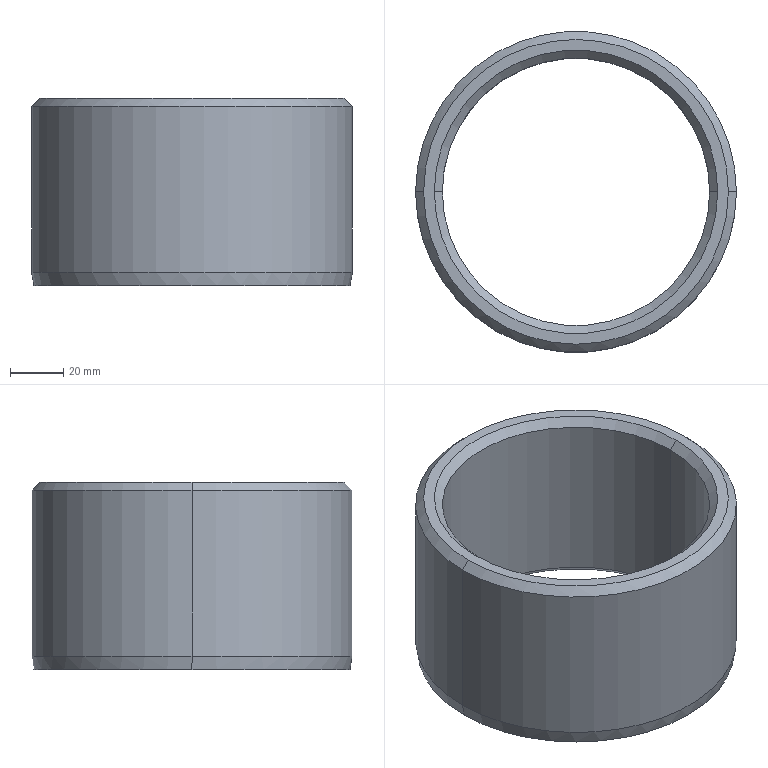Part | SolidWorks | features Chamfer 2, Extrusion 1 | 1 solid | 14 faces | box 120 x 120 x 70 mm | volume 236524 mm3 | cone 8 | cylinder 4 | plane 2 | commonest cylinder face diameters 100 x2 120 x2
STEP:
#1=CARTESIAN_POINT('',(-59.118,0.,-35.));
#2=VERTEX_POINT('',#1);
#3=CARTESIAN_POINT('',(59.118,0.,-35.));
#4=VERTEX_POINT('',#3);
#5=CARTESIAN_POINT('',(0.,0.,-35.));
#6=DIRECTION('',(0.,0.,-1.));
#7=DIRECTION('',(1.,0.,0.));
#8=AXIS2_PLACEMENT_3D('',#5,#6,#7);
#9=CIRCLE('',#8,59.118);
#10=EDGE_CURVE('',#2,#4,#9,.T.);
#11=ORIENTED_EDGE('',*,*,#10,.F.);
#12=CARTESIAN_POINT('',(-60.,0.,-30.));
#13=VERTEX_POINT('',#12);
#14=CARTESIAN_POINT('',(-60.,0.,-30.));
#15=DIRECTION('',(-0.1736,0.,0.9848));
#16=VECTOR('',#15,1000.);
#17=LINE('',#14,#16);
#18=EDGE_CURVE('',#2,#13,#17,.T.);
#19=ORIENTED_EDGE('',*,*,#18,.T.);
#20=CARTESIAN_POINT('',(60.,0.,-30.));
#21=VERTEX_POINT('',#20);
#22=CARTESIAN_POINT('',(0.,0.,-30.));
#23=DIRECTION('',(0.,0.,1.));
#24=DIRECTION('',(1.,0.,0.));
#25=AXIS2_PLACEMENT_3D('',#22,#23,#24);
#26=CIRCLE('',#25,60.);
#27=EDGE_CURVE('',#21,#13,#26,.T.);
#28=ORIENTED_EDGE('',*,*,#27,.F.);
#29=CARTESIAN_POINT('',(60.,0.,-30.));
#30=DIRECTION('',(0.1736,0.,0.9848));
#31=VECTOR('',#30,1000.);
#32=LINE('',#29,#31);
#33=EDGE_CURVE('',#4,#21,#32,.T.);
#34=ORIENTED_EDGE('',*,*,#33,.F.);
#35=EDGE_LOOP('',(#11,#19,#28,#34));
#36=FACE_OUTER_BOUND('',#35,.T.);
#37=CARTESIAN_POINT('',(0.,0.,-30.));
#38=DIRECTION('',(0.,0.,1.));
#39=DIRECTION('',(1.,0.,0.));
#40=AXIS2_PLACEMENT_3D('',#37,#38,#39);
#41=CONICAL_SURFACE('',#40,60.,0.1745);
#42=ADVANCED_FACE('',(#36),#41,.T.);
#43=CARTESIAN_POINT('',(57.,0.,35.));
#44=VERTEX_POINT('',#43);
#45=CARTESIAN_POINT('',(-57.,0.,35.));
#46=VERTEX_POINT('',#45);
#47=CARTESIAN_POINT('',(0.,0.,35.));
#48=DIRECTION('',(0.,0.,1.));
#49=DIRECTION('',(1.,0.,0.));
#50=AXIS2_PLACEMENT_3D('',#47,#48,#49);
#51=CIRCLE('',#50,57.);
#52=EDGE_CURVE('',#44,#46,#51,.T.);
#53=ORIENTED_EDGE('',*,*,#52,.F.);
#54=CARTESIAN_POINT('',(60.,0.,32.));
#55=VERTEX_POINT('',#54);
#56=CARTESIAN_POINT('',(57.,0.,35.));
#57=DIRECTION('',(0.7071,0.,-0.7071));
#58=VECTOR('',#57,1000.);
#59=LINE('',#56,#58);
#60=EDGE_CURVE('',#44,#55,#59,.T.);
#61=ORIENTED_EDGE('',*,*,#60,.T.);
#62=CARTESIAN_POINT('',(-60.,0.,32.));
#63=VERTEX_POINT('',#62);
#64=CARTESIAN_POINT('',(0.,0.,32.));
#65=DIRECTION('',(0.,0.,-1.));
#66=DIRECTION('',(1.,0.,0.));
#67=AXIS2_PLACEMENT_3D('',#64,#65,#66);
#68=CIRCLE('',#67,60.);
#69=EDGE_CURVE('',#63,#55,#68,.T.);
#70=ORIENTED_EDGE('',*,*,#69,.F.);
#71=CARTESIAN_POINT('',(-57.,0.,35.));
#72=DIRECTION('',(-0.7071,0.,-0.7071));
#73=VECTOR('',#72,1000.);
#74=LINE('',#71,#73);
#75=EDGE_CURVE('',#46,#63,#74,.T.);
#76=ORIENTED_EDGE('',*,*,#75,.F.);
#77=EDGE_LOOP('',(#53,#61,#70,#76));
#78=FACE_OUTER_BOUND('',#77,.T.);
#79=CARTESIAN_POINT('',(0.,0.,35.));
#80=DIRECTION('',(0.,0.,-1.));
#81=DIRECTION('',(-1.,0.,0.));
#82=AXIS2_PLACEMENT_3D('',#79,#80,#81);
#83=CONICAL_SURFACE('',#82,57.,0.7854);
#84=ADVANCED_FACE('',(#78),#83,.T.);
#85=CARTESIAN_POINT('',(-50.,0.,32.));
#86=VERTEX_POINT('',#85);
#87=CARTESIAN_POINT('',(50.,0.,32.));
#88=VERTEX_POINT('',#87);
#89=CARTESIAN_POINT('',(0.,0.,32.));
#90=DIRECTION('',(0.,0.,1.));
#91=DIRECTION('',(1.,0.,0.));
#92=AXIS2_PLACEMENT_3D('',#89,#90,#91);
#93=CIRCLE('',#92,50.);
#94=EDGE_CURVE('',#86,#88,#93,.T.);
#95=ORIENTED_EDGE('',*,*,#94,.F.);
#96=CARTESIAN_POINT('',(-53.,0.,35.));
#97=VERTEX_POINT('',#96);
#98=CARTESIAN_POINT('',(-50.,0.,32.));
#99=DIRECTION('',(-0.7071,0.,0.7071));
#100=VECTOR('',#99,1000.);
#101=LINE('',#98,#100);
#102=EDGE_CURVE('',#86,#97,#101,.T.);
#103=ORIENTED_EDGE('',*,*,#102,.T.);
#104=CARTESIAN_POINT('',(53.,0.,35.));
#105=VERTEX_POINT('',#104);
#106=CARTESIAN_POINT('',(0.,0.,35.));
#107=DIRECTION('',(0.,0.,-1.));
#108=DIRECTION('',(1.,0.,0.));
#109=AXIS2_PLACEMENT_3D('',#106,#107,#108);
#110=CIRCLE('',#109,53.);
#111=EDGE_CURVE('',#105,#97,#110,.T.);
#112=ORIENTED_EDGE('',*,*,#111,.F.);
#113=CARTESIAN_POINT('',(50.,0.,32.));
#114=DIRECTION('',(0.7071,0.,0.7071));
#115=VECTOR('',#114,1000.);
#116=LINE('',#113,#115);
#117=EDGE_CURVE('',#88,#105,#116,.T.);
#118=ORIENTED_EDGE('',*,*,#117,.F.);
#119=EDGE_LOOP('',(#95,#103,#112,#118));
#120=FACE_OUTER_BOUND('',#119,.T.);
#121=CARTESIAN_POINT('',(0.,0.,32.));
#122=DIRECTION('',(0.,0.,1.));
#123=DIRECTION('',(1.,0.,0.));
#124=AXIS2_PLACEMENT_3D('',#121,#122,#123);
#125=CONICAL_SURFACE('',#124,50.,0.7854);
#126=ADVANCED_FACE('',(#120),#125,.F.);
#127=CARTESIAN_POINT('',(50.,0.,-32.));
#128=VERTEX_POINT('',#127);
#129=CARTESIAN_POINT('',(-50.,0.,-32.));
#130=VERTEX_POINT('',#129);
#131=CARTESIAN_POINT('',(0.,0.,-32.));
#132=DIRECTION('',(0.,0.,-1.));
#133=DIRECTION('',(1.,0.,0.));
#134=AXIS2_PLACEMENT_3D('',#131,#132,#133);
#135=CIRCLE('',#134,50.);
#136=EDGE_CURVE('',#128,#130,#135,.T.);
#137=ORIENTED_EDGE('',*,*,#136,.F.);
#138=CARTESIAN_POINT('',(53.,0.,-35.));
#139=VERTEX_POINT('',#138);
#140=CARTESIAN_POINT('',(53.,0.,-35.));
#141=DIRECTION('',(0.7071,0.,-0.7071));
#142=VECTOR('',#141,1000.);
#143=LINE('',#140,#142);
#144=EDGE_CURVE('',#128,#139,#143,.T.);
#145=ORIENTED_EDGE('',*,*,#144,.T.);
#146=CARTESIAN_POINT('',(-53.,0.,-35.));
#147=VERTEX_POINT('',#146);
#148=CARTESIAN_POINT('',(0.,0.,-35.));
#149=DIRECTION('',(0.,0.,1.));
#150=DIRECTION('',(1.,0.,0.));
#151=AXIS2_PLACEMENT_3D('',#148,#149,#150);
#152=CIRCLE('',#151,53.);
#153=EDGE_CURVE('',#147,#139,#152,.T.);
#154=ORIENTED_EDGE('',*,*,#153,.F.);
#155=CARTESIAN_POINT('',(-53.,0.,-35.));
#156=DIRECTION('',(-0.7071,0.,-0.7071));
#157=VECTOR('',#156,1000.);
#158=LINE('',#155,#157);
#159=EDGE_CURVE('',#130,#147,#158,.T.);
#160=ORIENTED_EDGE('',*,*,#159,.F.);
#161=EDGE_LOOP('',(#137,#145,#154,#160));
#162=FACE_OUTER_BOUND('',#161,.T.);
#163=CARTESIAN_POINT('',(0.,0.,-35.));
#164=DIRECTION('',(0.,0.,-1.));
#165=DIRECTION('',(-1.,0.,0.));
#166=AXIS2_PLACEMENT_3D('',#163,#164,#165);
#167=CONICAL_SURFACE('',#166,53.,0.7854);
#168=ADVANCED_FACE('',(#162),#167,.F.);
#169=ORIENTED_EDGE('',*,*,#94,.T.);
#170=CARTESIAN_POINT('',(50.,0.,35.));
#171=DIRECTION('',(0.,0.,-1.));
#172=VECTOR('',#171,1000.);
#173=LINE('',#170,#172);
#174=EDGE_CURVE('',#88,#128,#173,.T.);
#175=ORIENTED_EDGE('',*,*,#174,.T.);
#176=ORIENTED_EDGE('',*,*,#136,.T.);
#177=CARTESIAN_POINT('',(-50.,0.,35.));
#178=DIRECTION('',(0.,0.,-1.));
#179=VECTOR('',#178,1000.);
#180=LINE('',#177,#179);
#181=EDGE_CURVE('',#86,#130,#180,.T.);
#182=ORIENTED_EDGE('',*,*,#181,.F.);
#183=EDGE_LOOP('',(#169,#175,#176,#182));
#184=FACE_OUTER_BOUND('',#183,.T.);
#185=CARTESIAN_POINT('',(0.,0.,35.));
#186=DIRECTION('',(0.,0.,-1.));
#187=DIRECTION('',(-1.,0.,0.));
#188=AXIS2_PLACEMENT_3D('',#185,#186,#187);
#189=CYLINDRICAL_SURFACE('',#188,50.);
#190=ADVANCED_FACE('',(#184),#189,.F.);
#191=ORIENTED_EDGE('',*,*,#69,.T.);
#192=CARTESIAN_POINT('',(60.,0.,35.));
#193=DIRECTION('',(0.,0.,-1.));
#194=VECTOR('',#193,1000.);
#195=LINE('',#192,#194);
#196=EDGE_CURVE('',#55,#21,#195,.T.);
#197=ORIENTED_EDGE('',*,*,#196,.T.);
#198=ORIENTED_EDGE('',*,*,#27,.T.);
#199=CARTESIAN_POINT('',(-60.,0.,35.));
#200=DIRECTION('',(0.,0.,-1.));
#201=VECTOR('',#200,1000.);
#202=LINE('',#199,#201);
#203=EDGE_CURVE('',#63,#13,#202,.T.);
#204=ORIENTED_EDGE('',*,*,#203,.F.);
#205=EDGE_LOOP('',(#191,#197,#198,#204));
#206=FACE_OUTER_BOUND('',#205,.T.);
#207=CARTESIAN_POINT('',(0.,0.,35.));
#208=DIRECTION('',(0.,0.,-1.));
#209=DIRECTION('',(-1.,0.,0.));
#210=AXIS2_PLACEMENT_3D('',#207,#208,#209);
#211=CYLINDRICAL_SURFACE('',#210,60.);
#212=ADVANCED_FACE('',(#206),#211,.T.);
#213=ORIENTED_EDGE('',*,*,#111,.T.);
#214=CARTESIAN_POINT('',(0.,0.,35.));
#215=DIRECTION('',(0.,0.,-1.));
#216=DIRECTION('',(1.,0.,0.));
#217=AXIS2_PLACEMENT_3D('',#214,#215,#216);
#218=CIRCLE('',#217,53.);
#219=EDGE_CURVE('',#97,#105,#218,.T.);
#220=ORIENTED_EDGE('',*,*,#219,.T.);
#221=EDGE_LOOP('',(#213,#220));
#222=FACE_BOUND('',#221,.T.);
#223=CARTESIAN_POINT('',(0.,0.,35.));
#224=DIRECTION('',(0.,0.,1.));
#225=DIRECTION('',(1.,0.,0.));
#226=AXIS2_PLACEMENT_3D('',#223,#224,#225);
#227=CIRCLE('',#226,57.);
#228=EDGE_CURVE('',#46,#44,#227,.T.);
#229=ORIENTED_EDGE('',*,*,#228,.T.);
#230=ORIENTED_EDGE('',*,*,#52,.T.);
#231=EDGE_LOOP('',(#229,#230));
#232=FACE_OUTER_BOUND('',#231,.T.);
#233=CARTESIAN_POINT('',(0.,0.,35.));
#234=DIRECTION('',(0.,0.,1.));
#235=DIRECTION('',(1.,0.,0.));
#236=AXIS2_PLACEMENT_3D('',#233,#234,#235);
#237=PLANE('',#236);
#238=ADVANCED_FACE('',(#222,#232),#237,.T.);
#239=CARTESIAN_POINT('',(0.,0.,-35.));
#240=DIRECTION('',(0.,0.,-1.));
#241=DIRECTION('',(1.,0.,0.));
#242=AXIS2_PLACEMENT_3D('',#239,#240,#241);
#243=CIRCLE('',#242,59.118);
#244=EDGE_CURVE('',#4,#2,#243,.T.);
#245=ORIENTED_EDGE('',*,*,#244,.T.);
#246=ORIENTED_EDGE('',*,*,#10,.T.);
#247=EDGE_LOOP('',(#245,#246));
#248=FACE_OUTER_BOUND('',#247,.T.);
#249=ORIENTED_EDGE('',*,*,#153,.T.);
#250=CARTESIAN_POINT('',(0.,0.,-35.));
#251=DIRECTION('',(0.,0.,1.));
#252=DIRECTION('',(1.,0.,0.));
#253=AXIS2_PLACEMENT_3D('',#250,#251,#252);
#254=CIRCLE('',#253,53.);
#255=EDGE_CURVE('',#139,#147,#254,.T.);
#256=ORIENTED_EDGE('',*,*,#255,.T.);
#257=EDGE_LOOP('',(#249,#256));
#258=FACE_BOUND('',#257,.T.);
#259=CARTESIAN_POINT('',(0.,0.,-35.));
#260=DIRECTION('',(0.,0.,1.));
#261=DIRECTION('',(1.,0.,0.));
#262=AXIS2_PLACEMENT_3D('',#259,#260,#261);
#263=PLANE('',#262);
#264=ADVANCED_FACE('',(#248,#258),#263,.F.);
#265=ORIENTED_EDGE('',*,*,#196,.F.);
#266=CARTESIAN_POINT('',(0.,0.,32.));
#267=DIRECTION('',(0.,0.,-1.));
#268=DIRECTION('',(1.,0.,0.));
#269=AXIS2_PLACEMENT_3D('',#266,#267,#268);
#270=CIRCLE('',#269,60.);
#271=EDGE_CURVE('',#55,#63,#270,.T.);
#272=ORIENTED_EDGE('',*,*,#271,.T.);
#273=ORIENTED_EDGE('',*,*,#203,.T.);
#274=CARTESIAN_POINT('',(0.,0.,-30.));
#275=DIRECTION('',(0.,0.,1.));
#276=DIRECTION('',(1.,0.,0.));
#277=AXIS2_PLACEMENT_3D('',#274,#275,#276);
#278=CIRCLE('',#277,60.);
#279=EDGE_CURVE('',#13,#21,#278,.T.);
#280=ORIENTED_EDGE('',*,*,#279,.T.);
#281=EDGE_LOOP('',(#265,#272,#273,#280));
#282=FACE_OUTER_BOUND('',#281,.T.);
#283=CARTESIAN_POINT('',(0.,0.,35.));
#284=DIRECTION('',(0.,0.,-1.));
#285=DIRECTION('',(-1.,0.,0.));
#286=AXIS2_PLACEMENT_3D('',#283,#284,#285);
#287=CYLINDRICAL_SURFACE('',#286,60.);
#288=ADVANCED_FACE('',(#282),#287,.T.);
#289=ORIENTED_EDGE('',*,*,#174,.F.);
#290=CARTESIAN_POINT('',(0.,0.,32.));
#291=DIRECTION('',(0.,0.,1.));
#292=DIRECTION('',(1.,0.,0.));
#293=AXIS2_PLACEMENT_3D('',#290,#291,#292);
#294=CIRCLE('',#293,50.);
#295=EDGE_CURVE('',#88,#86,#294,.T.);
#296=ORIENTED_EDGE('',*,*,#295,.T.);
#297=ORIENTED_EDGE('',*,*,#181,.T.);
#298=CARTESIAN_POINT('',(0.,0.,-32.));
#299=DIRECTION('',(0.,0.,-1.));
#300=DIRECTION('',(1.,0.,0.));
#301=AXIS2_PLACEMENT_3D('',#298,#299,#300);
#302=CIRCLE('',#301,50.);
#303=EDGE_CURVE('',#130,#128,#302,.T.);
#304=ORIENTED_EDGE('',*,*,#303,.T.);
#305=EDGE_LOOP('',(#289,#296,#297,#304));
#306=FACE_OUTER_BOUND('',#305,.T.);
#307=CARTESIAN_POINT('',(0.,0.,35.));
#308=DIRECTION('',(0.,0.,-1.));
#309=DIRECTION('',(-1.,0.,0.));
#310=AXIS2_PLACEMENT_3D('',#307,#308,#309);
#311=CYLINDRICAL_SURFACE('',#310,50.);
#312=ADVANCED_FACE('',(#306),#311,.F.);
#313=ORIENTED_EDGE('',*,*,#144,.F.);
#314=ORIENTED_EDGE('',*,*,#303,.F.);
#315=ORIENTED_EDGE('',*,*,#159,.T.);
#316=ORIENTED_EDGE('',*,*,#255,.F.);
#317=EDGE_LOOP('',(#313,#314,#315,#316));
#318=FACE_OUTER_BOUND('',#317,.T.);
#319=CARTESIAN_POINT('',(0.,0.,-35.));
#320=DIRECTION('',(0.,0.,-1.));
#321=DIRECTION('',(-1.,0.,0.));
#322=AXIS2_PLACEMENT_3D('',#319,#320,#321);
#323=CONICAL_SURFACE('',#322,53.,0.7854);
#324=ADVANCED_FACE('',(#318),#323,.F.);
#325=ORIENTED_EDGE('',*,*,#102,.F.);
#326=ORIENTED_EDGE('',*,*,#295,.F.);
#327=ORIENTED_EDGE('',*,*,#117,.T.);
#328=ORIENTED_EDGE('',*,*,#219,.F.);
#329=EDGE_LOOP('',(#325,#326,#327,#328));
#330=FACE_OUTER_BOUND('',#329,.T.);
#331=CARTESIAN_POINT('',(0.,0.,32.));
#332=DIRECTION('',(0.,0.,1.));
#333=DIRECTION('',(1.,0.,0.));
#334=AXIS2_PLACEMENT_3D('',#331,#332,#333);
#335=CONICAL_SURFACE('',#334,50.,0.7854);
#336=ADVANCED_FACE('',(#330),#335,.F.);
#337=ORIENTED_EDGE('',*,*,#60,.F.);
#338=ORIENTED_EDGE('',*,*,#228,.F.);
#339=ORIENTED_EDGE('',*,*,#75,.T.);
#340=ORIENTED_EDGE('',*,*,#271,.F.);
#341=EDGE_LOOP('',(#337,#338,#339,#340));
#342=FACE_OUTER_BOUND('',#341,.T.);
#343=CARTESIAN_POINT('',(0.,0.,35.));
#344=DIRECTION('',(0.,0.,-1.));
#345=DIRECTION('',(-1.,0.,0.));
#346=AXIS2_PLACEMENT_3D('',#343,#344,#345);
#347=CONICAL_SURFACE('',#346,57.,0.7854);
#348=ADVANCED_FACE('',(#342),#347,.T.);
#349=ORIENTED_EDGE('',*,*,#18,.F.);
#350=ORIENTED_EDGE('',*,*,#244,.F.);
#351=ORIENTED_EDGE('',*,*,#33,.T.);
#352=ORIENTED_EDGE('',*,*,#279,.F.);
#353=EDGE_LOOP('',(#349,#350,#351,#352));
#354=FACE_OUTER_BOUND('',#353,.T.);
#355=CARTESIAN_POINT('',(0.,0.,-30.));
#356=DIRECTION('',(0.,0.,1.));
#357=DIRECTION('',(1.,0.,0.));
#358=AXIS2_PLACEMENT_3D('',#355,#356,#357);
#359=CONICAL_SURFACE('',#358,60.,0.1745);
#360=ADVANCED_FACE('',(#354),#359,.T.);
#361=CLOSED_SHELL('',(#42,#84,#126,#168,#190,#212,#238,#264,#288,#312,#324,#336,#348,#360));
#362=MANIFOLD_SOLID_BREP('',#361);
#363=CARTESIAN_POINT('',(0.,0.,0.));
#364=DIRECTION('',(0.,0.,1.));
#365=DIRECTION('',(1.,0.,0.));
#366=AXIS2_PLACEMENT_3D('',#363,#364,#365);
#367=(LENGTH_UNIT()NAMED_UNIT(*)SI_UNIT(.MILLI.,.METRE.));
#368=UNCERTAINTY_MEASURE_WITH_UNIT(LENGTH_MEASURE(0.00001),#367,'','');
#369=(NAMED_UNIT(*)PLANE_ANGLE_UNIT()SI_UNIT($,.RADIAN.));
#370=(NAMED_UNIT(*)SI_UNIT($,.STERADIAN.)SOLID_ANGLE_UNIT());
#371=(GEOMETRIC_REPRESENTATION_CONTEXT(3)GLOBAL_UNCERTAINTY_ASSIGNED_CONTEXT((#368))GLOBAL_UNIT_ASSIGNED_CONTEXT((#367,#369,#370))REPRESENTATION_CONTEXT('',''));
#372=ADVANCED_BREP_SHAPE_REPRESENTATION('',(#362,#366),#371);